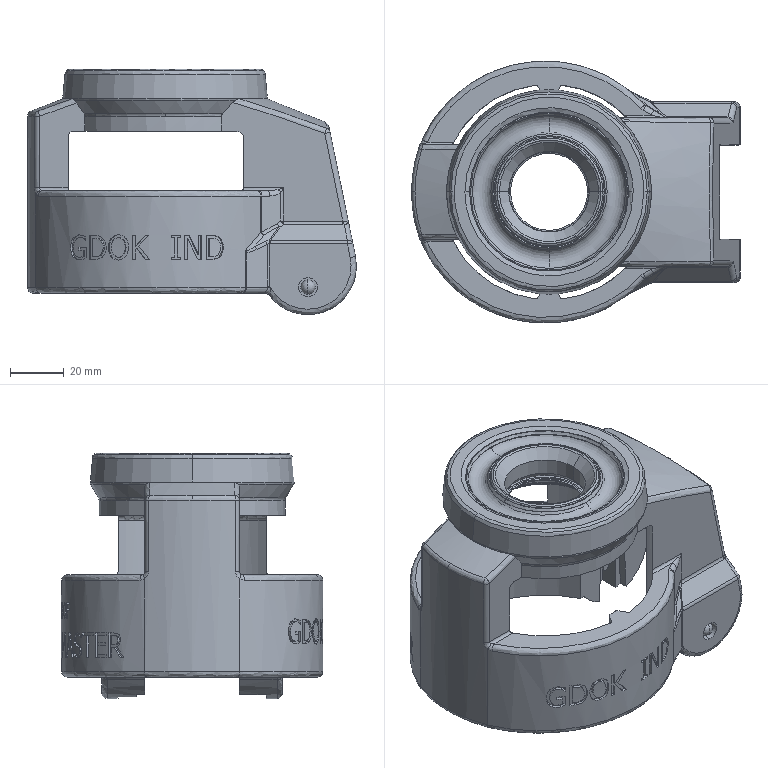Part | SolidWorks | features BaseBody 1 | 1 solid | 650 faces | box 122 x 97.04 x 91 mm | volume 221114 mm3 | spline 265 | plane 216 | cylinder 103 | cone 37 | torus 23 | sphere 6 | commonest cylinder face diameters 4 x28 98.54 x24 2 x12 100.54 x12 12.437 x5 3 x4